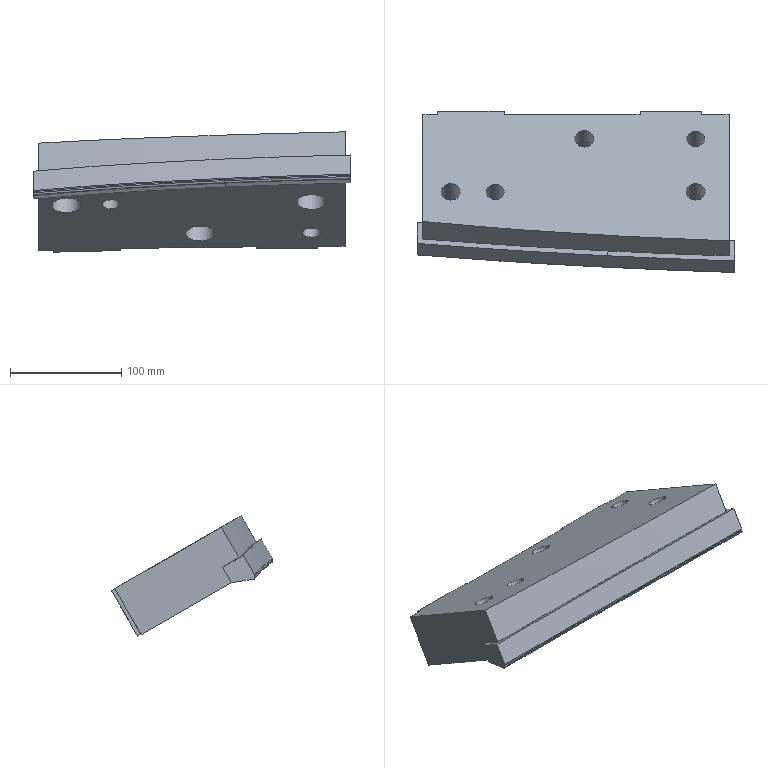Part | NX | features MAIN_BODY 2 | 1 solid | 41 faces | box 285 x 144.79 x 108.065 mm | volume 1500904 mm3 | plane 19 | spline 13 | cylinder 9 | commonest cylinder face diameters 17 x3 26 x3 16 x2 5.004 x1